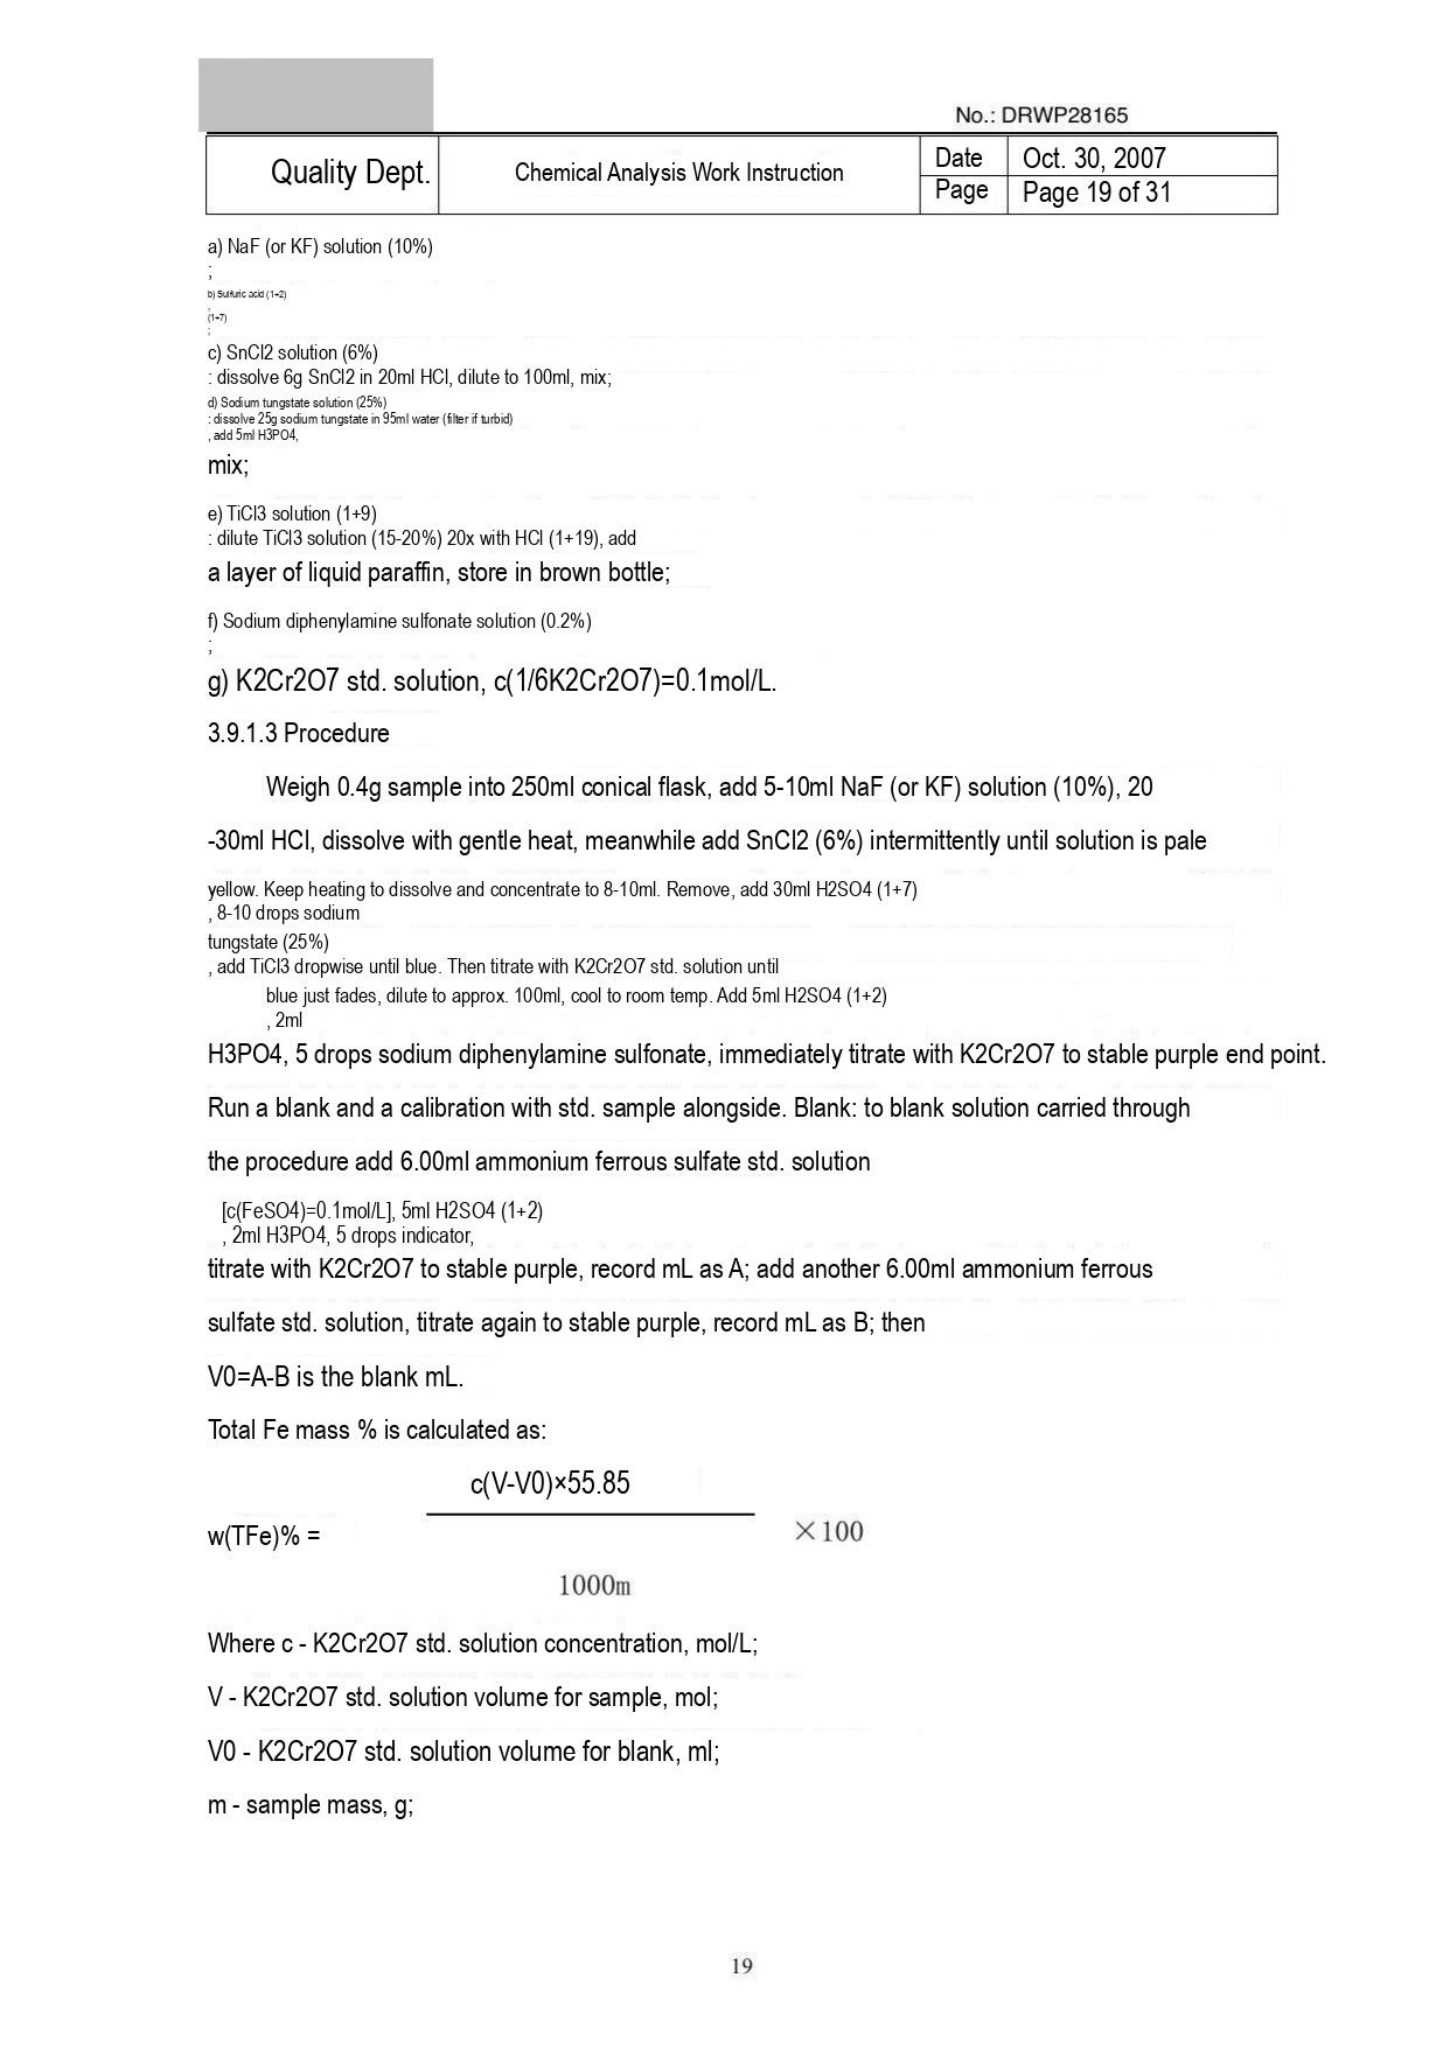No.: DRWP28165

| Quality Dept. | Chemical Analysis Work Instruction | Date | Oct. 30, 2007 |
|---|---|---|---|
| | | Page | Page 19 of 31 |

a) NaF (or KF) solution (10%)
;
b) Sulfuric acid (1+2)
;
(1+7)
;
c) SnCl2 solution (6%)
: dissolve 6g SnCl2 in 20ml HCl, dilute to 100ml, mix;
d) Sodium tungstate solution (25%)
: dissolve 25g sodium tungstate in 95ml water (filter if turbid)
, add 5ml H3PO4,
mix;
e) TiCl3 solution (1+9)
: dilute TiCl3 solution (15-20%) 20x with HCl (1+19), add
a layer of liquid paraffin, store in brown bottle;
f) Sodium diphenylamine sulfonate solution (0.2%)
;
g) K2Cr2O7 std. solution, c(1/6K2Cr2O7)=0.1mol/L.

3.9.1.3 Procedure

Weigh 0.4g sample into 250ml conical flask, add 5-10ml NaF (or KF) solution (10%), 20
-30ml HCl, dissolve with gentle heat, meanwhile add SnCl2 (6%) intermittently until solution is pale
yellow. Keep heating to dissolve and concentrate to 8-10ml. Remove, add 30ml H2SO4 (1+7)
, 8-10 drops sodium
tungstate (25%)
, add TiCl3 dropwise until blue. Then titrate with K2Cr2O7 std. solution until
blue just fades, dilute to approx. 100ml, cool to room temp. Add 5ml H2SO4 (1+2)
, 2ml
H3PO4, 5 drops sodium diphenylamine sulfonate, immediately titrate with K2Cr2O7 to stable purple end point.
Run a blank and a calibration with std. sample alongside. Blank: to blank solution carried through
the procedure add 6.00ml ammonium ferrous sulfate std. solution
[c(FeSO4)=0.1mol/L], 5ml H2SO4 (1+2)
, 2ml H3PO4, 5 drops indicator,
titrate with K2Cr2O7 to stable purple, record mL as A; add another 6.00ml ammonium ferrous
sulfate std. solution, titrate again to stable purple, record mL as B; then
V0=A-B is the blank mL.

Total Fe mass % is calculated as:

w(TFe)% = c(V-V0)×55.85 / 1000m ×100

Where c - K2Cr2O7 std. solution concentration, mol/L;
V - K2Cr2O7 std. solution volume for sample, mol;
V0 - K2Cr2O7 std. solution volume for blank, ml;
m - sample mass, g;

19
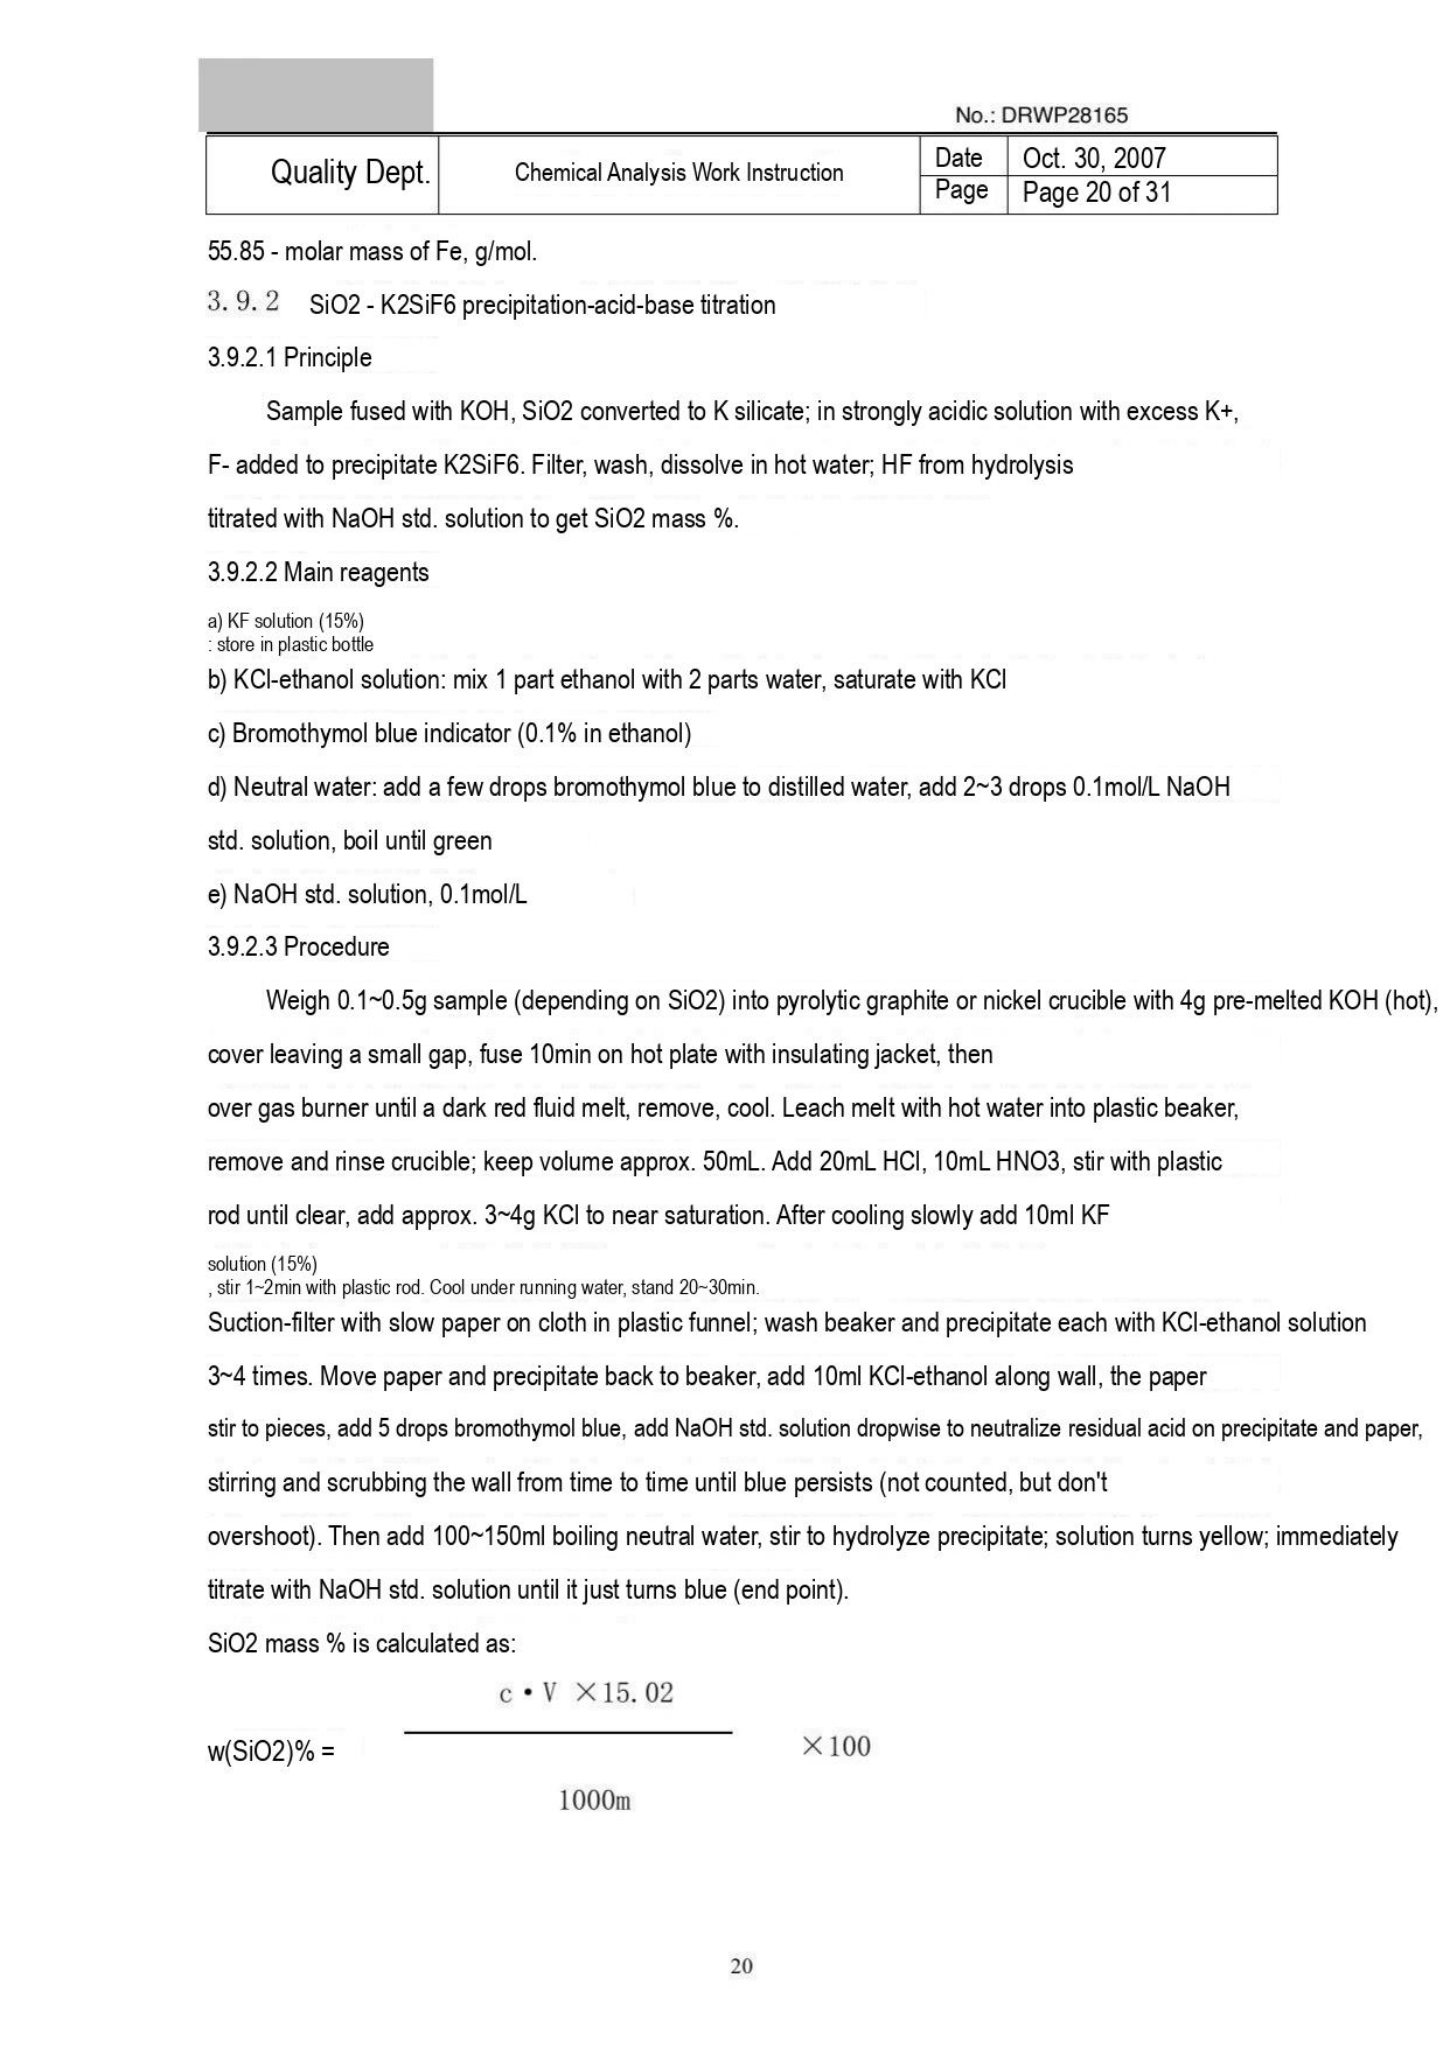No.: DRWP28165

| Quality Dept. | Chemical Analysis Work Instruction | Date | Oct. 30, 2007 |
|---|---|---|---|
| | | Page | Page 20 of 31 |

55.85 - molar mass of Fe, g/mol.

3. 9. 2 SiO2 - K2SiF6 precipitation-acid-base titration

3.9.2.1 Principle

Sample fused with KOH, SiO2 converted to K silicate; in strongly acidic solution with excess K+, F- added to precipitate K2SiF6. Filter, wash, dissolve in hot water; HF from hydrolysis titrated with NaOH std. solution to get SiO2 mass %.

3.9.2.2 Main reagents

a) KF solution (15%)
: store in plastic bottle

b) KCl-ethanol solution: mix 1 part ethanol with 2 parts water, saturate with KCl

c) Bromothymol blue indicator (0.1% in ethanol)

d) Neutral water: add a few drops bromothymol blue to distilled water, add 2~3 drops 0.1mol/L NaOH std. solution, boil until green

e) NaOH std. solution, 0.1mol/L

3.9.2.3 Procedure

Weigh 0.1~0.5g sample (depending on SiO2) into pyrolytic graphite or nickel crucible with 4g pre-melted KOH (hot), cover leaving a small gap, fuse 10min on hot plate with insulating jacket, then over gas burner until a dark red fluid melt, remove, cool. Leach melt with hot water into plastic beaker, remove and rinse crucible; keep volume approx. 50mL. Add 20mL HCl, 10mL HNO3, stir with plastic rod until clear, add approx. 3~4g KCl to near saturation. After cooling slowly add 10ml KF solution (15%)
, stir 1~2min with plastic rod. Cool under running water, stand 20~30min.
Suction-filter with slow paper on cloth in plastic funnel; wash beaker and precipitate each with KCl-ethanol solution 3~4 times. Move paper and precipitate back to beaker, add 10ml KCl-ethanol along wall, the paper stir to pieces, add 5 drops bromothymol blue, add NaOH std. solution dropwise to neutralize residual acid on precipitate and paper, stirring and scrubbing the wall from time to time until blue persists (not counted, but don't overshoot). Then add 100~150ml boiling neutral water, stir to hydrolyze precipitate; solution turns yellow; immediately titrate with NaOH std. solution until it just turns blue (end point).

SiO2 mass % is calculated as:

w(SiO2)% = (c • V ×15. 02) / (1000m) ×100

20
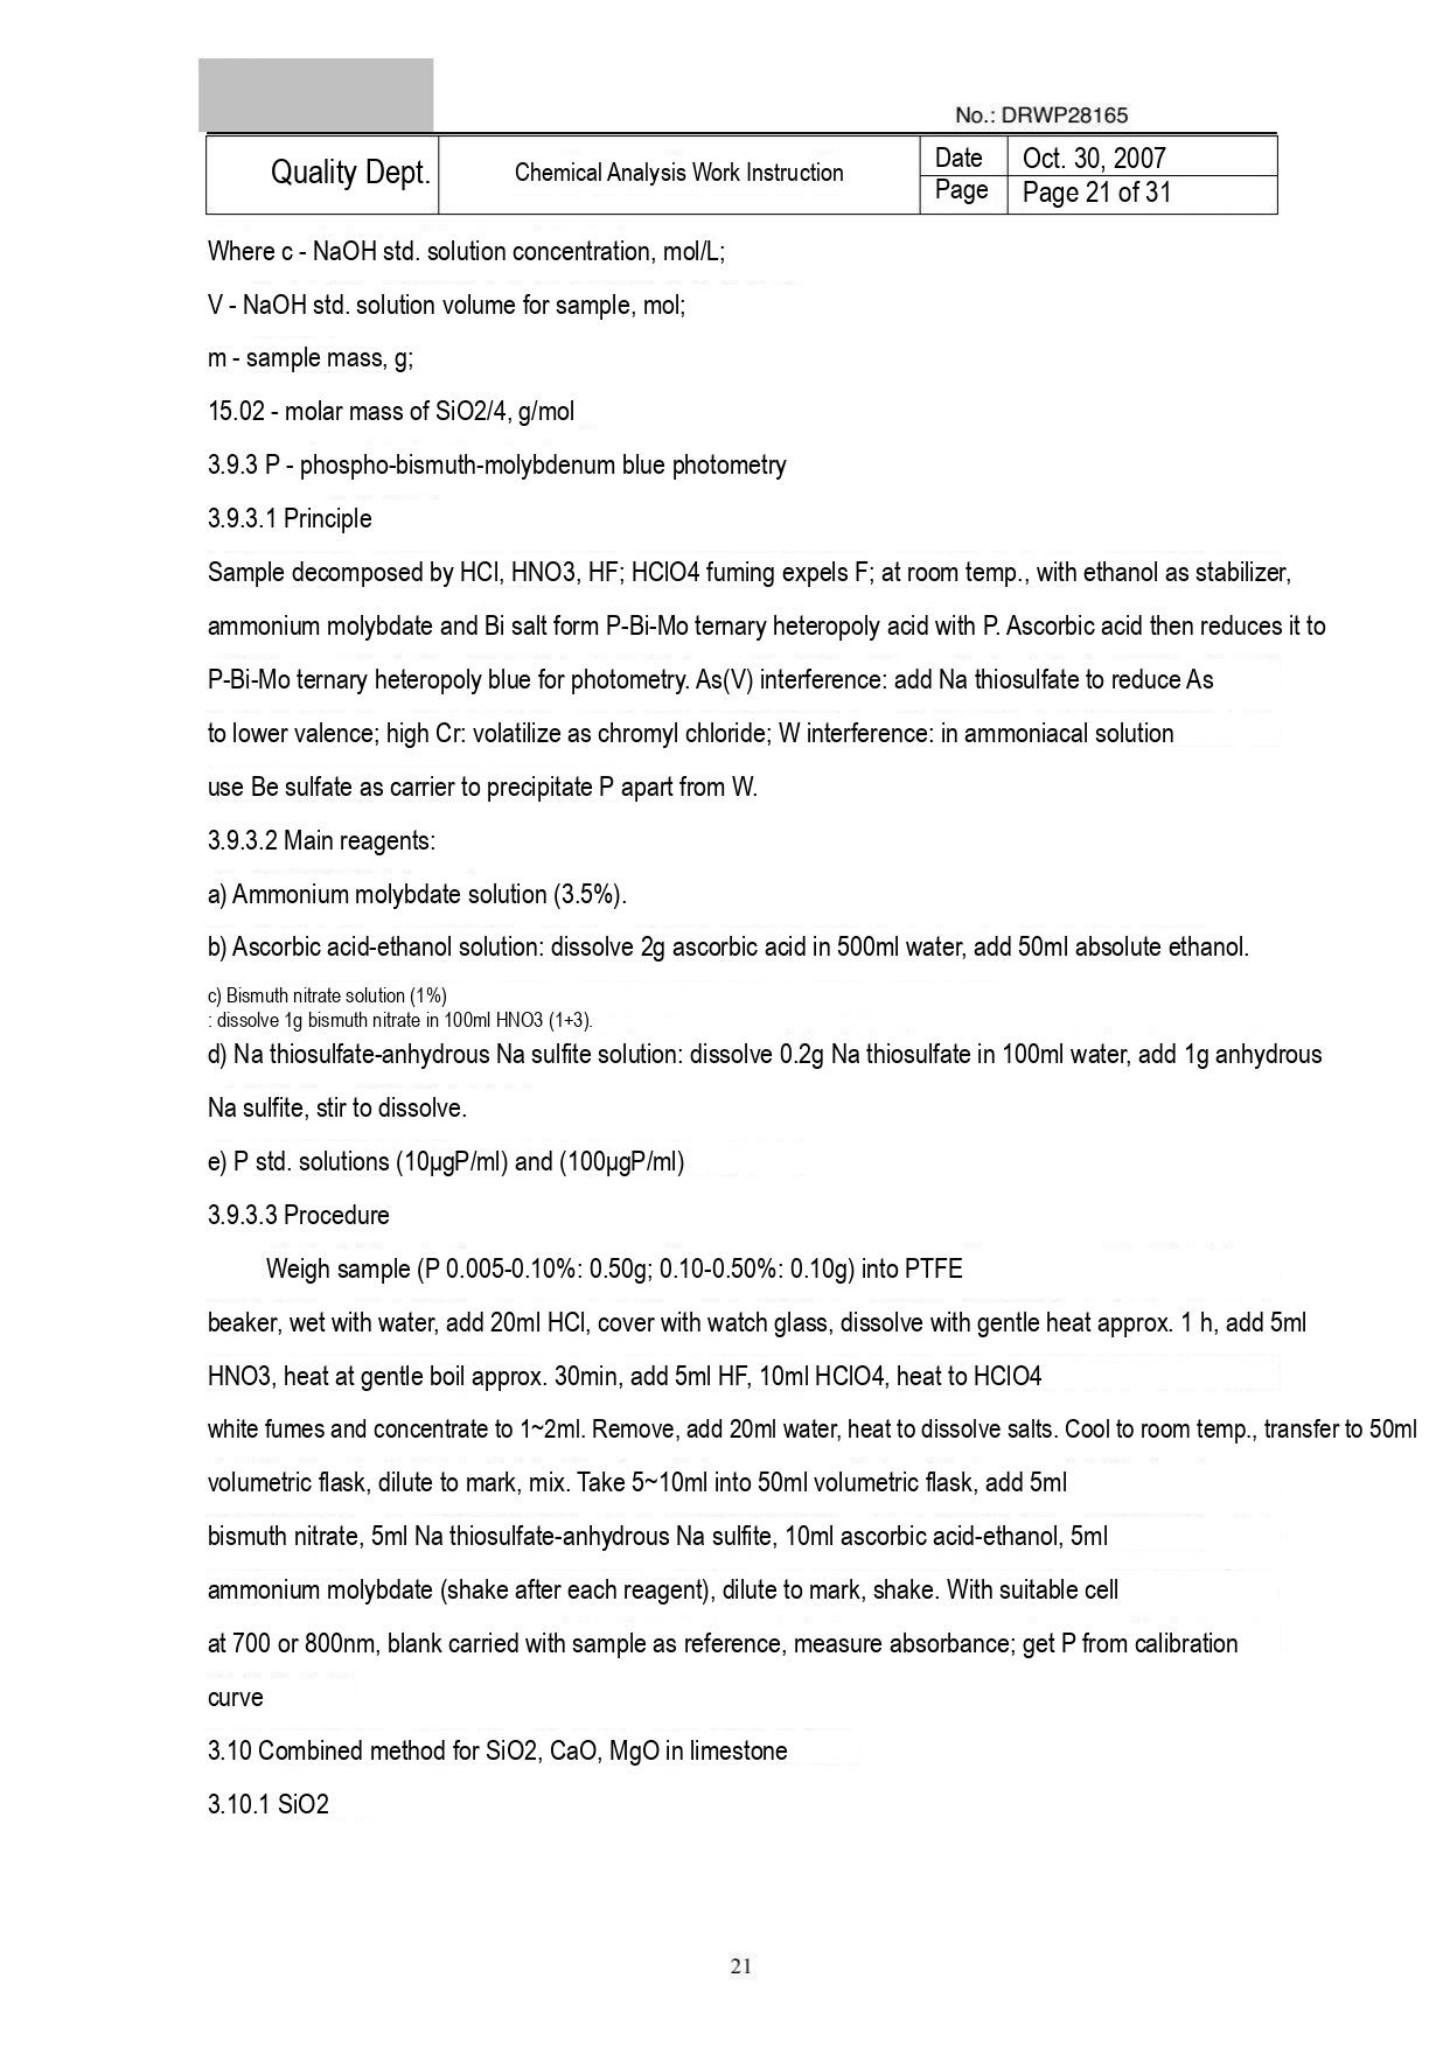No.: DRWP28165

| Quality Dept. | Chemical Analysis Work Instruction | Date | Oct. 30, 2007 |
|---|---|---|---|
| | | Page | Page 21 of 31 |

Where c - NaOH std. solution concentration, mol/L;

V - NaOH std. solution volume for sample, mol;

m - sample mass, g;

15.02 - molar mass of SiO2/4, g/mol

3.9.3 P - phospho-bismuth-molybdenum blue photometry

3.9.3.1 Principle

Sample decomposed by HCl, HNO3, HF; HClO4 fuming expels F; at room temp., with ethanol as stabilizer, ammonium molybdate and Bi salt form P-Bi-Mo ternary heteropoly acid with P. Ascorbic acid then reduces it to P-Bi-Mo ternary heteropoly blue for photometry. As(V) interference: add Na thiosulfate to reduce As to lower valence; high Cr: volatilize as chromyl chloride; W interference: in ammoniacal solution use Be sulfate as carrier to precipitate P apart from W.

3.9.3.2 Main reagents:

a) Ammonium molybdate solution (3.5%).

b) Ascorbic acid-ethanol solution: dissolve 2g ascorbic acid in 500ml water, add 50ml absolute ethanol.

c) Bismuth nitrate solution (1%)
: dissolve 1g bismuth nitrate in 100ml HNO3 (1+3).

d) Na thiosulfate-anhydrous Na sulfite solution: dissolve 0.2g Na thiosulfate in 100ml water, add 1g anhydrous Na sulfite, stir to dissolve.

e) P std. solutions (10µgP/ml) and (100µgP/ml)

3.9.3.3 Procedure

Weigh sample (P 0.005-0.10%: 0.50g; 0.10-0.50%: 0.10g) into PTFE beaker, wet with water, add 20ml HCl, cover with watch glass, dissolve with gentle heat approx. 1 h, add 5ml HNO3, heat at gentle boil approx. 30min, add 5ml HF, 10ml HClO4, heat to HClO4 white fumes and concentrate to 1~2ml. Remove, add 20ml water, heat to dissolve salts. Cool to room temp., transfer to 50ml volumetric flask, dilute to mark, mix. Take 5~10ml into 50ml volumetric flask, add 5ml bismuth nitrate, 5ml Na thiosulfate-anhydrous Na sulfite, 10ml ascorbic acid-ethanol, 5ml ammonium molybdate (shake after each reagent), dilute to mark, shake. With suitable cell at 700 or 800nm, blank carried with sample as reference, measure absorbance; get P from calibration curve

3.10 Combined method for SiO2, CaO, MgO in limestone

3.10.1 SiO2

21
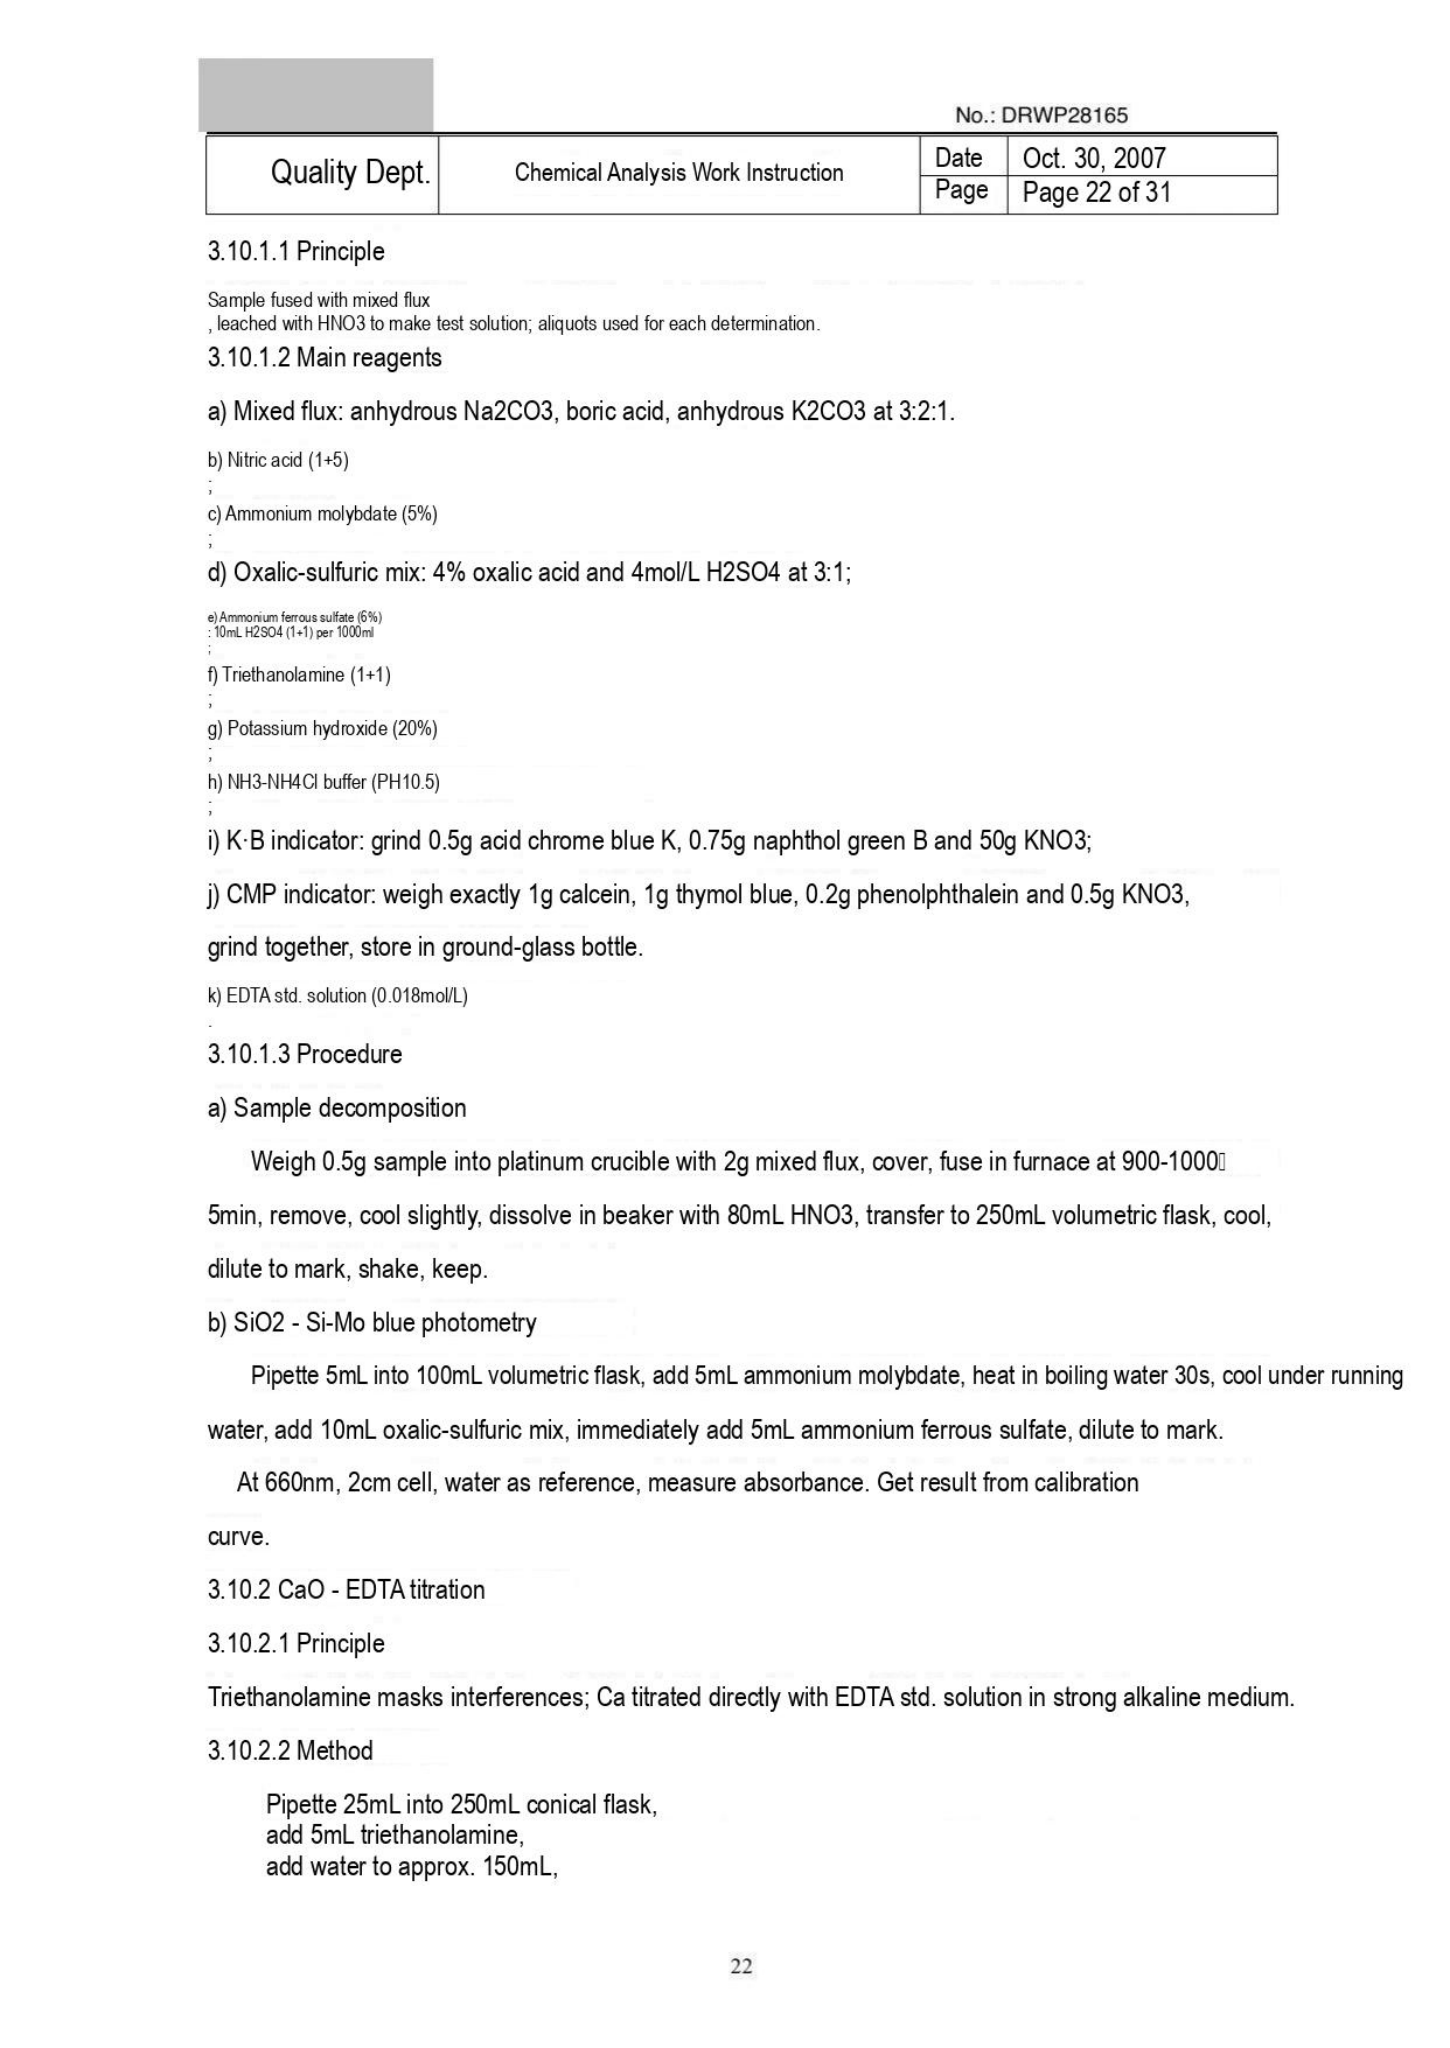No.: DRWP28165

| Quality Dept. | Chemical Analysis Work Instruction | Date | Oct. 30, 2007 |
|---|---|---|---|
| | | Page | Page 22 of 31 |

3.10.1.1 Principle

Sample fused with mixed flux
, leached with HNO3 to make test solution; aliquots used for each determination.

3.10.1.2 Main reagents

a) Mixed flux: anhydrous Na2CO3, boric acid, anhydrous K2CO3 at 3:2:1.

b) Nitric acid (1+5)
;
c) Ammonium molybdate (5%)
;
d) Oxalic-sulfuric mix: 4% oxalic acid and 4mol/L H2SO4 at 3:1;

e) Ammonium ferrous sulfate (6%)
: 10mL H2SO4 (1+1) per 1000ml
;
f) Triethanolamine (1+1)
;
g) Potassium hydroxide (20%)
;
h) NH3-NH4Cl buffer (PH10.5)
;
i) K·B indicator: grind 0.5g acid chrome blue K, 0.75g naphthol green B and 50g KNO3;

j) CMP indicator: weigh exactly 1g calcein, 1g thymol blue, 0.2g phenolphthalein and 0.5g KNO3, grind together, store in ground-glass bottle.

k) EDTA std. solution (0.018mol/L)
.

3.10.1.3 Procedure

a) Sample decomposition

Weigh 0.5g sample into platinum crucible with 2g mixed flux, cover, fuse in furnace at 900-1000 5min, remove, cool slightly, dissolve in beaker with 80mL HNO3, transfer to 250mL volumetric flask, cool, dilute to mark, shake, keep.

b) SiO2 - Si-Mo blue photometry

Pipette 5mL into 100mL volumetric flask, add 5mL ammonium molybdate, heat in boiling water 30s, cool under running water, add 10mL oxalic-sulfuric mix, immediately add 5mL ammonium ferrous sulfate, dilute to mark.

At 660nm, 2cm cell, water as reference, measure absorbance. Get result from calibration curve.

3.10.2 CaO - EDTA titration

3.10.2.1 Principle

Triethanolamine masks interferences; Ca titrated directly with EDTA std. solution in strong alkaline medium.

3.10.2.2 Method

Pipette 25mL into 250mL conical flask,
add 5mL triethanolamine,
add water to approx. 150mL,

22
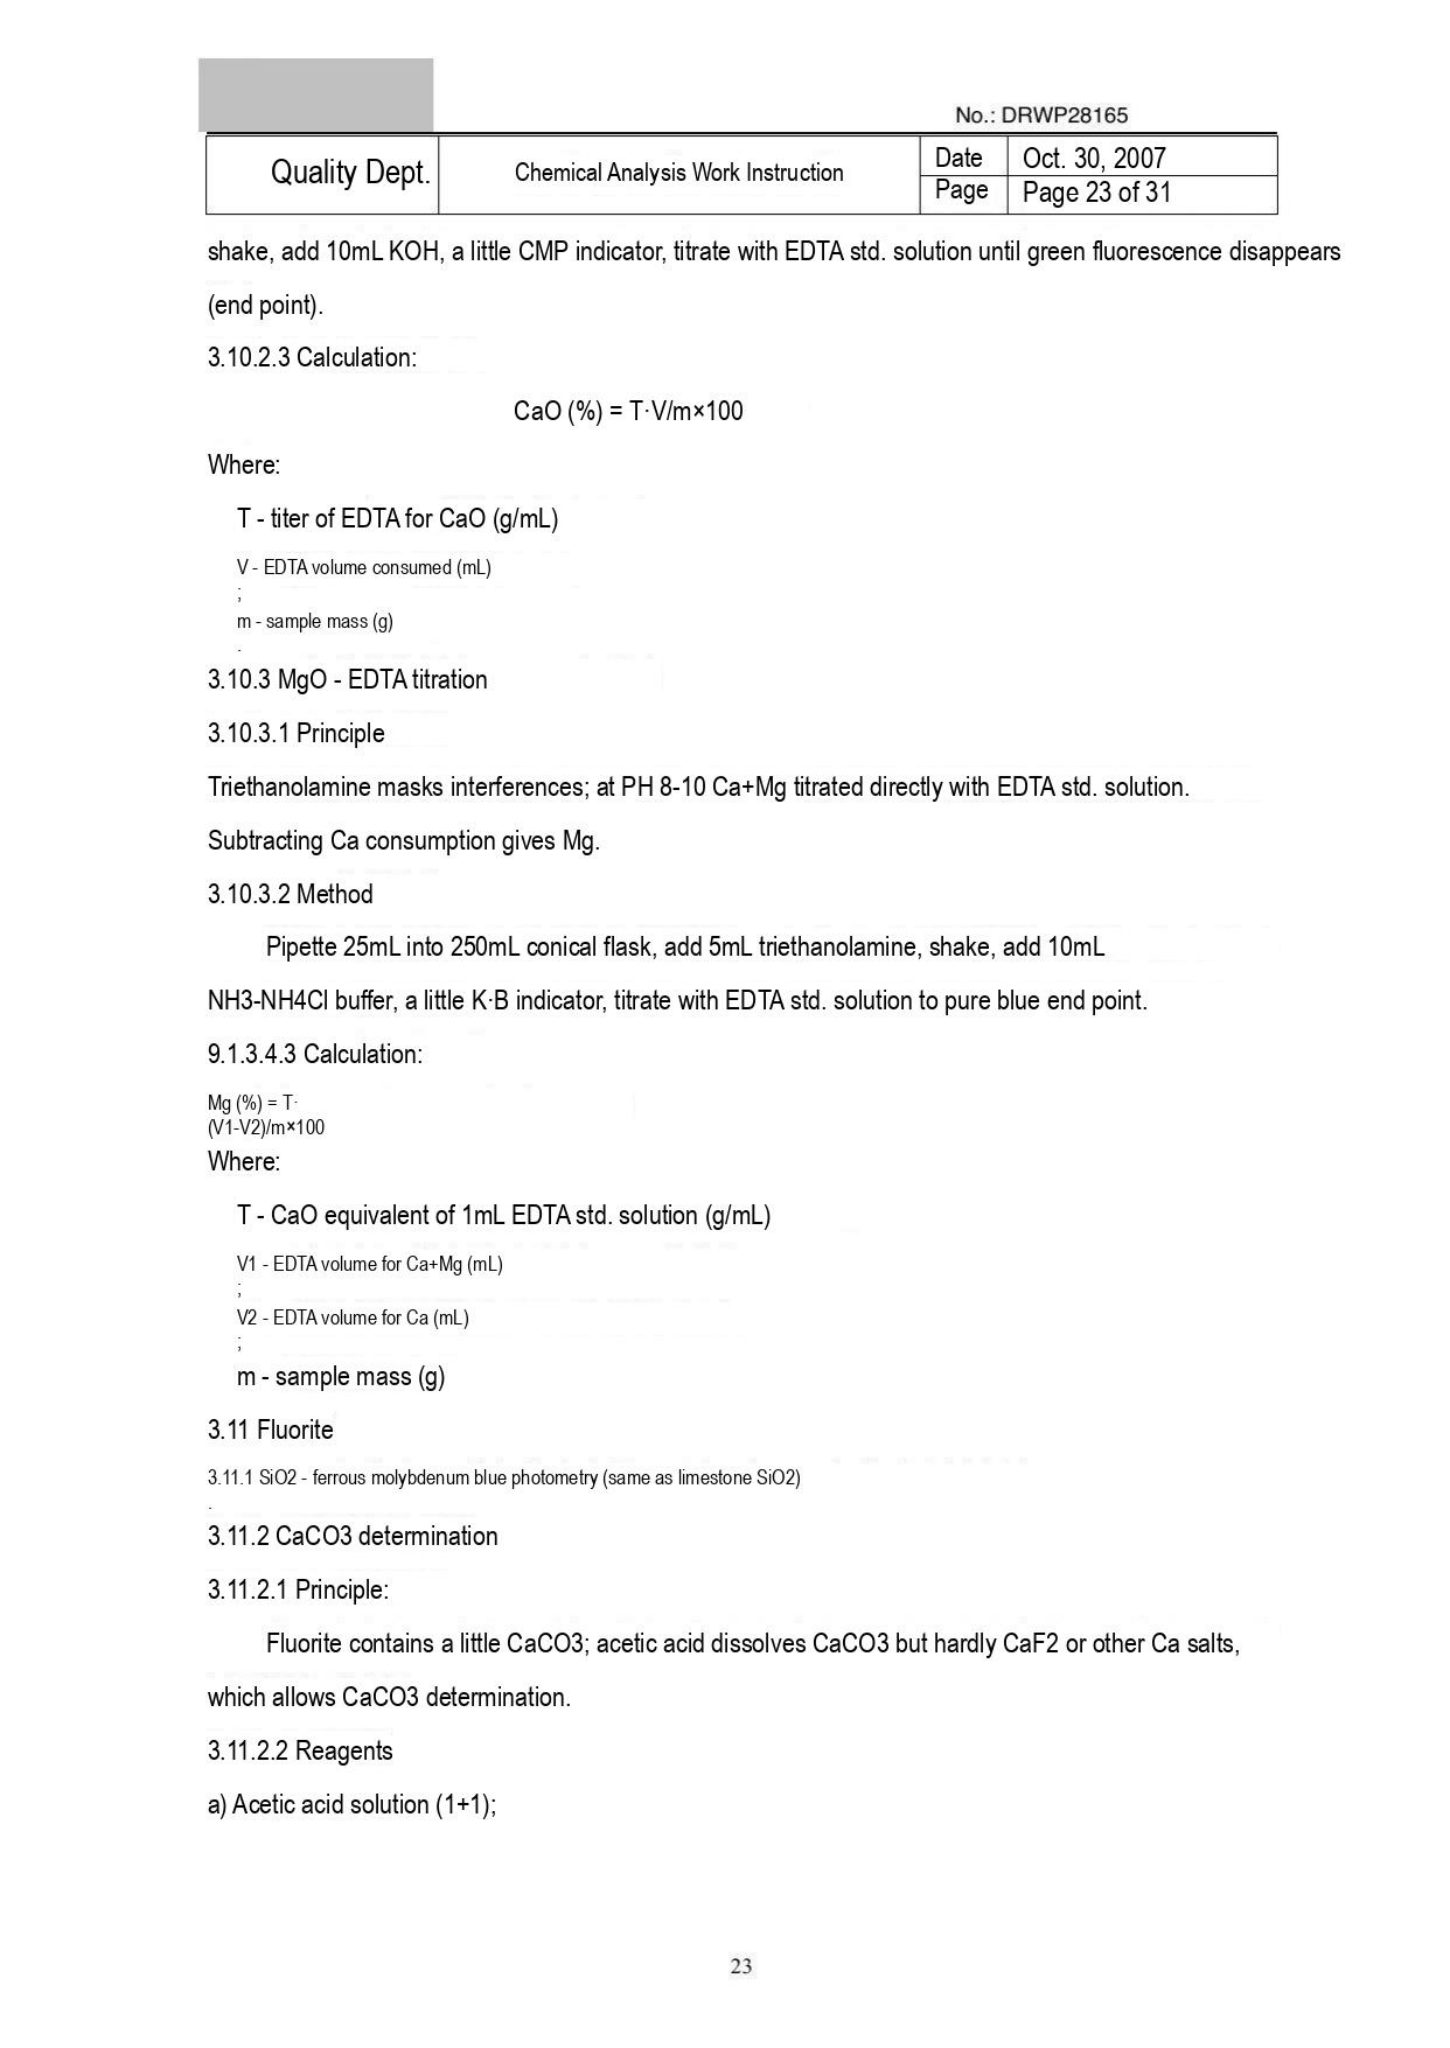No.: DRWP28165

| Quality Dept. | Chemical Analysis Work Instruction | Date | Oct. 30, 2007 |
|---|---|---|---|
| | | Page | Page 23 of 31 |

shake, add 10mL KOH, a little CMP indicator, titrate with EDTA std. solution until green fluorescence disappears (end point).

3.10.2.3 Calculation:

CaO (%) = T·V/m×100

Where:

T - titer of EDTA for CaO (g/mL)

V - EDTA volume consumed (mL)
;
m - sample mass (g)
.

3.10.3 MgO - EDTA titration

3.10.3.1 Principle

Triethanolamine masks interferences; at PH 8-10 Ca+Mg titrated directly with EDTA std. solution. Subtracting Ca consumption gives Mg.

3.10.3.2 Method

Pipette 25mL into 250mL conical flask, add 5mL triethanolamine, shake, add 10mL NH3-NH4Cl buffer, a little K·B indicator, titrate with EDTA std. solution to pure blue end point.

9.1.3.4.3 Calculation:

Mg (%) = T·
(V1-V2)/m×100

Where:

T - CaO equivalent of 1mL EDTA std. solution (g/mL)

V1 - EDTA volume for Ca+Mg (mL)
;
V2 - EDTA volume for Ca (mL)
;
m - sample mass (g)

3.11 Fluorite

3.11.1 SiO2 - ferrous molybdenum blue photometry (same as limestone SiO2)
.

3.11.2 CaCO3 determination

3.11.2.1 Principle:

Fluorite contains a little CaCO3; acetic acid dissolves CaCO3 but hardly CaF2 or other Ca salts, which allows CaCO3 determination.

3.11.2.2 Reagents

a) Acetic acid solution (1+1);

23
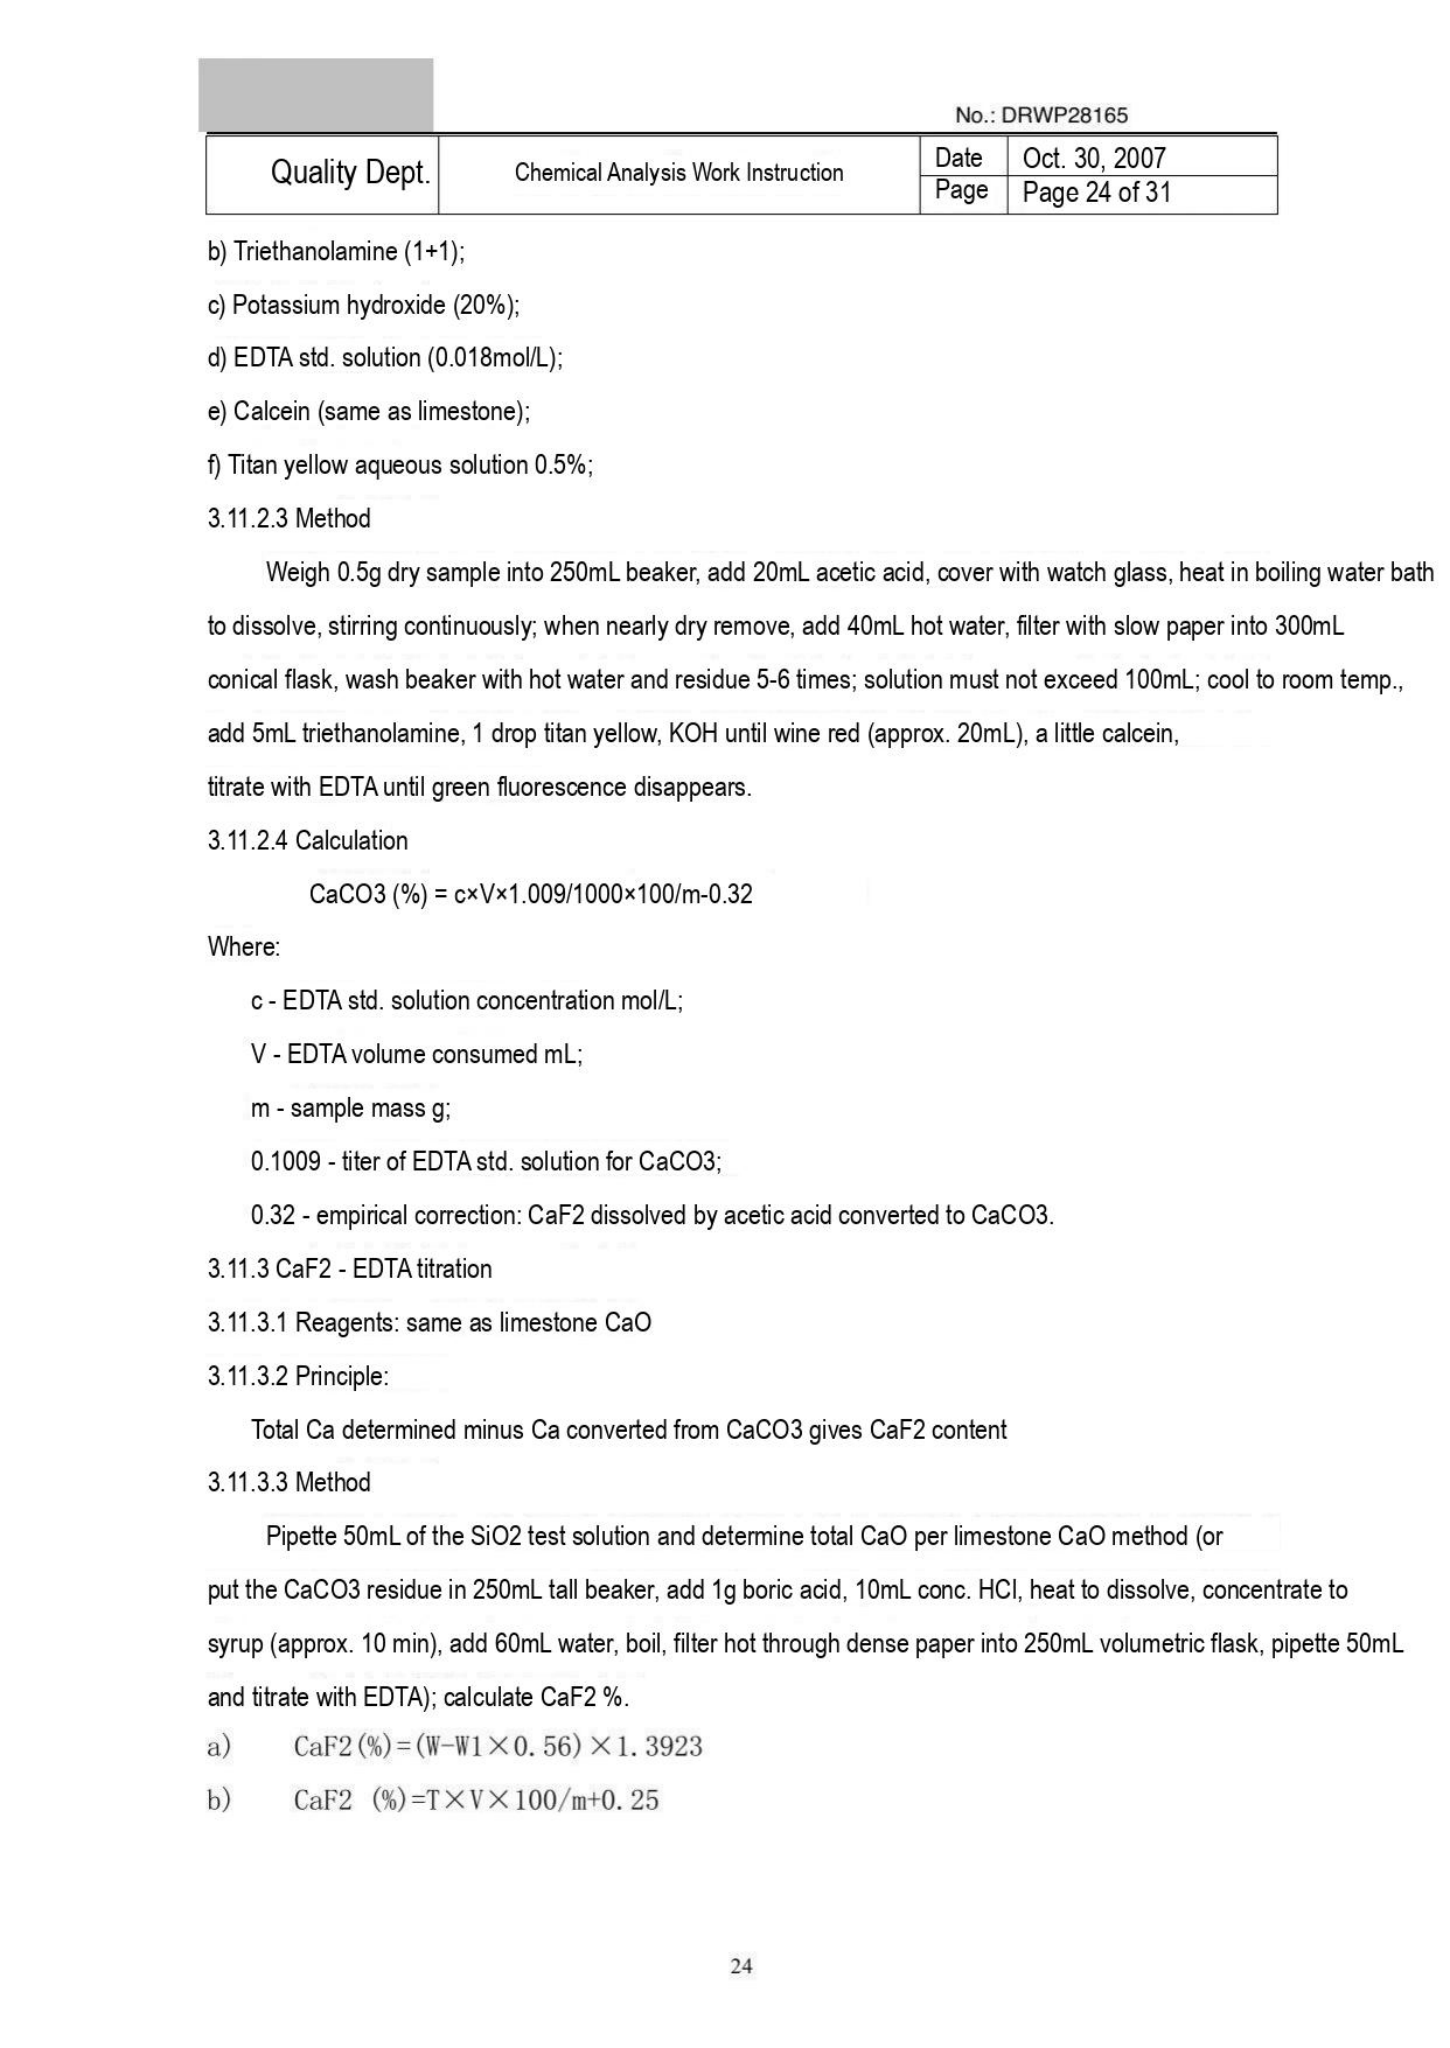No.: DRWP28165

| Quality Dept. | Chemical Analysis Work Instruction | Date | Oct. 30, 2007 |
|---|---|---|---|
| | | Page | Page 24 of 31 |

b) Triethanolamine (1+1);

c) Potassium hydroxide (20%);

d) EDTA std. solution (0.018mol/L);

e) Calcein (same as limestone);

f) Titan yellow aqueous solution 0.5%;

3.11.2.3 Method

Weigh 0.5g dry sample into 250mL beaker, add 20mL acetic acid, cover with watch glass, heat in boiling water bath to dissolve, stirring continuously; when nearly dry remove, add 40mL hot water, filter with slow paper into 300mL conical flask, wash beaker with hot water and residue 5-6 times; solution must not exceed 100mL; cool to room temp., add 5mL triethanolamine, 1 drop titan yellow, KOH until wine red (approx. 20mL), a little calcein, titrate with EDTA until green fluorescence disappears.

3.11.2.4 Calculation

CaCO3 (%) = c×V×1.009/1000×100/m-0.32

Where:

c - EDTA std. solution concentration mol/L;

V - EDTA volume consumed mL;

m - sample mass g;

0.1009 - titer of EDTA std. solution for CaCO3;

0.32 - empirical correction: CaF2 dissolved by acetic acid converted to CaCO3.

3.11.3 CaF2 - EDTA titration

3.11.3.1 Reagents: same as limestone CaO

3.11.3.2 Principle:

Total Ca determined minus Ca converted from CaCO3 gives CaF2 content

3.11.3.3 Method

Pipette 50mL of the SiO2 test solution and determine total CaO per limestone CaO method (or put the CaCO3 residue in 250mL tall beaker, add 1g boric acid, 10mL conc. HCl, heat to dissolve, concentrate to syrup (approx. 10 min), add 60mL water, boil, filter hot through dense paper into 250mL volumetric flask, pipette 50mL and titrate with EDTA); calculate CaF2 %.

a) CaF2 (%) = (W-W1×0.56)×1.3923

b) CaF2 (%) =T×V×100/m+0.25

24